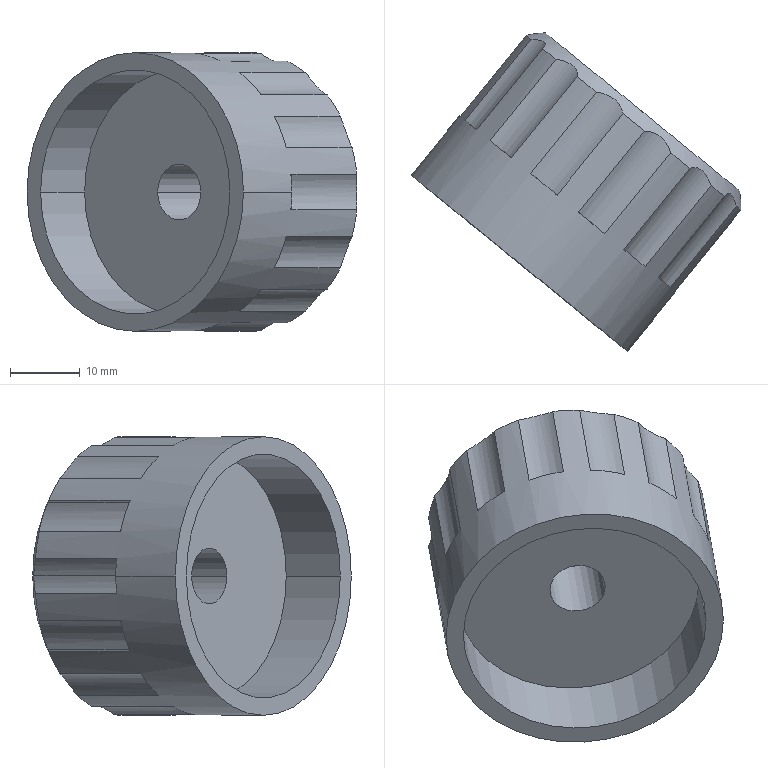Part | SolidWorks | features BaseBody 1 | 1 solid | 48 faces | box 47.315 x 45.699 x 40 mm | volume 23891 mm3 | cylinder 27 | plane 19 | cone 2 | commonest cylinder face diameters 10 x19 5 x2 8 x2 35 x2 40 x2